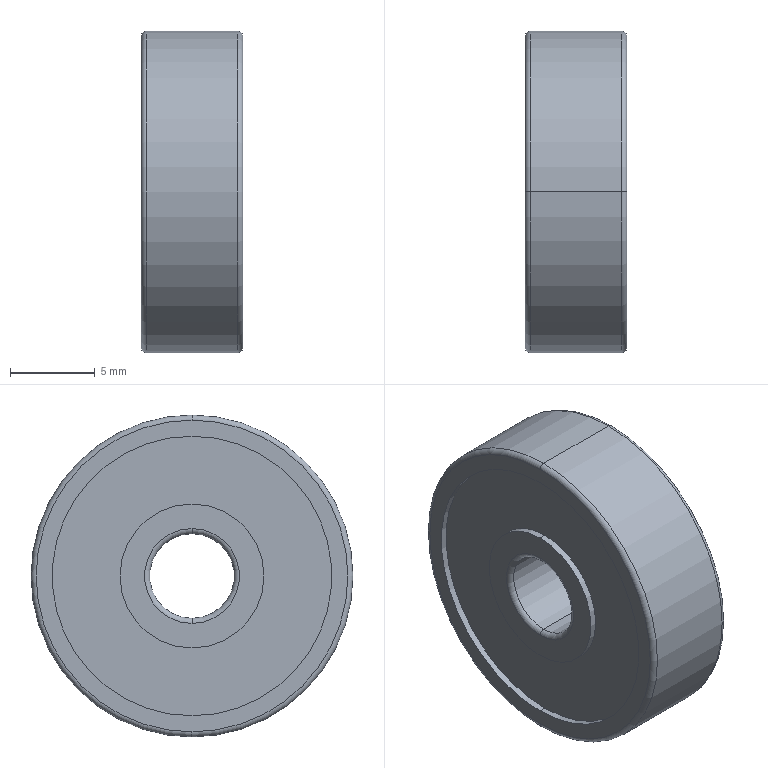Part | SolidWorks | features RefAxis 6, 3DProfileFeature 2, Revolution 1 | 1 solid | 26 faces | box 6 x 19 x 19 mm | volume 1455 mm3 | cylinder 12 | torus 8 | plane 6 | commonest cylinder face diameters 8.5 x4 16.5 x4 5 x2 19 x2
STEP:
#1=CARTESIAN_POINT('',(5.7,0.,9.5));
#2=VERTEX_POINT('',#1);
#3=CARTESIAN_POINT('',(5.7,0.,-9.5));
#4=VERTEX_POINT('',#3);
#5=CARTESIAN_POINT('',(5.7,0.,0.));
#6=DIRECTION('',(-1.,0.,0.));
#7=DIRECTION('',(0.,0.,1.));
#8=AXIS2_PLACEMENT_3D('',#5,#6,#7);
#9=CIRCLE('',#8,9.5);
#10=EDGE_CURVE('',#2,#4,#9,.T.);
#11=ORIENTED_EDGE('',*,*,#10,.T.);
#12=CARTESIAN_POINT('',(0.3,0.,-9.5));
#13=VERTEX_POINT('',#12);
#14=CARTESIAN_POINT('',(5.7,0.,-9.5));
#15=DIRECTION('',(-1.,0.,0.));
#16=VECTOR('',#15,1000.);
#17=LINE('',#14,#16);
#18=EDGE_CURVE('',#4,#13,#17,.T.);
#19=ORIENTED_EDGE('',*,*,#18,.T.);
#20=CARTESIAN_POINT('',(0.3,0.,9.5));
#21=VERTEX_POINT('',#20);
#22=CARTESIAN_POINT('',(0.3,0.,0.));
#23=DIRECTION('',(-1.,0.,0.));
#24=DIRECTION('',(0.,0.,1.));
#25=AXIS2_PLACEMENT_3D('',#22,#23,#24);
#26=CIRCLE('',#25,9.5);
#27=EDGE_CURVE('',#21,#13,#26,.T.);
#28=ORIENTED_EDGE('',*,*,#27,.F.);
#29=CARTESIAN_POINT('',(5.7,0.,9.5));
#30=DIRECTION('',(-1.,0.,0.));
#31=VECTOR('',#30,1000.);
#32=LINE('',#29,#31);
#33=EDGE_CURVE('',#2,#21,#32,.T.);
#34=ORIENTED_EDGE('',*,*,#33,.F.);
#35=EDGE_LOOP('',(#11,#19,#28,#34));
#36=FACE_OUTER_BOUND('',#35,.T.);
#37=CARTESIAN_POINT('',(5.7,0.,0.));
#38=DIRECTION('',(-1.,0.,0.));
#39=DIRECTION('',(0.,0.,1.));
#40=AXIS2_PLACEMENT_3D('',#37,#38,#39);
#41=CYLINDRICAL_SURFACE('',#40,9.5);
#42=ADVANCED_FACE('',(#36),#41,.T.);
#43=CARTESIAN_POINT('',(6.,0.,9.2));
#44=VERTEX_POINT('',#43);
#45=CARTESIAN_POINT('',(6.,0.,-9.2));
#46=VERTEX_POINT('',#45);
#47=CARTESIAN_POINT('',(6.,0.,0.));
#48=DIRECTION('',(-1.,0.,0.));
#49=DIRECTION('',(0.,0.,1.));
#50=AXIS2_PLACEMENT_3D('',#47,#48,#49);
#51=CIRCLE('',#50,9.2);
#52=EDGE_CURVE('',#44,#46,#51,.T.);
#53=ORIENTED_EDGE('',*,*,#52,.T.);
#54=CARTESIAN_POINT('',(5.7,0.,-9.2));
#55=DIRECTION('',(0.,1.,0.));
#56=DIRECTION('',(0.,0.,1.));
#57=AXIS2_PLACEMENT_3D('',#54,#55,#56);
#58=CIRCLE('',#57,0.3);
#59=EDGE_CURVE('',#46,#4,#58,.T.);
#60=ORIENTED_EDGE('',*,*,#59,.T.);
#61=ORIENTED_EDGE('',*,*,#10,.F.);
#62=CARTESIAN_POINT('',(5.7,0.,9.2));
#63=DIRECTION('',(0.,-1.,0.));
#64=DIRECTION('',(0.,0.,-1.));
#65=AXIS2_PLACEMENT_3D('',#62,#63,#64);
#66=CIRCLE('',#65,0.3);
#67=EDGE_CURVE('',#44,#2,#66,.T.);
#68=ORIENTED_EDGE('',*,*,#67,.F.);
#69=EDGE_LOOP('',(#53,#60,#61,#68));
#70=FACE_OUTER_BOUND('',#69,.T.);
#71=CARTESIAN_POINT('',(5.7,0.,0.));
#72=DIRECTION('',(-1.,0.,0.));
#73=DIRECTION('',(0.,0.,1.));
#74=AXIS2_PLACEMENT_3D('',#71,#72,#73);
#75=TOROIDAL_SURFACE('',#74,9.2,0.3);
#76=ADVANCED_FACE('',(#70),#75,.T.);
#77=CARTESIAN_POINT('',(6.,0.,-8.25));
#78=VERTEX_POINT('',#77);
#79=CARTESIAN_POINT('',(6.,0.,8.25));
#80=VERTEX_POINT('',#79);
#81=CARTESIAN_POINT('',(6.,0.,0.));
#82=DIRECTION('',(-1.,0.,0.));
#83=DIRECTION('',(0.,0.,1.));
#84=AXIS2_PLACEMENT_3D('',#81,#82,#83);
#85=CIRCLE('',#84,8.25);
#86=EDGE_CURVE('',#78,#80,#85,.T.);
#87=ORIENTED_EDGE('',*,*,#86,.F.);
#88=CARTESIAN_POINT('',(5.602,0.,-8.25));
#89=VERTEX_POINT('',#88);
#90=CARTESIAN_POINT('',(5.7,0.,-8.25));
#91=DIRECTION('',(-1.,0.,0.));
#92=VECTOR('',#91,1000.);
#93=LINE('',#90,#92);
#94=EDGE_CURVE('',#78,#89,#93,.T.);
#95=ORIENTED_EDGE('',*,*,#94,.T.);
#96=CARTESIAN_POINT('',(5.602,0.,8.25));
#97=VERTEX_POINT('',#96);
#98=CARTESIAN_POINT('',(5.602,0.,0.));
#99=DIRECTION('',(-1.,0.,0.));
#100=DIRECTION('',(0.,0.,1.));
#101=AXIS2_PLACEMENT_3D('',#98,#99,#100);
#102=CIRCLE('',#101,8.25);
#103=EDGE_CURVE('',#89,#97,#102,.T.);
#104=ORIENTED_EDGE('',*,*,#103,.T.);
#105=CARTESIAN_POINT('',(5.7,0.,8.25));
#106=DIRECTION('',(-1.,0.,0.));
#107=VECTOR('',#106,1000.);
#108=LINE('',#105,#107);
#109=EDGE_CURVE('',#80,#97,#108,.T.);
#110=ORIENTED_EDGE('',*,*,#109,.F.);
#111=EDGE_LOOP('',(#87,#95,#104,#110));
#112=FACE_OUTER_BOUND('',#111,.T.);
#113=CARTESIAN_POINT('',(5.7,0.,0.));
#114=DIRECTION('',(-1.,0.,0.));
#115=DIRECTION('',(0.,0.,1.));
#116=AXIS2_PLACEMENT_3D('',#113,#114,#115);
#117=CYLINDRICAL_SURFACE('',#116,8.25);
#118=ADVANCED_FACE('',(#112),#117,.F.);
#119=CARTESIAN_POINT('',(6.,0.,4.25));
#120=VERTEX_POINT('',#119);
#121=CARTESIAN_POINT('',(6.,0.,-4.25));
#122=VERTEX_POINT('',#121);
#123=CARTESIAN_POINT('',(6.,0.,0.));
#124=DIRECTION('',(-1.,0.,0.));
#125=DIRECTION('',(0.,0.,1.));
#126=AXIS2_PLACEMENT_3D('',#123,#124,#125);
#127=CIRCLE('',#126,4.25);
#128=EDGE_CURVE('',#120,#122,#127,.T.);
#129=ORIENTED_EDGE('',*,*,#128,.T.);
#130=CARTESIAN_POINT('',(5.602,0.,-4.25));
#131=VERTEX_POINT('',#130);
#132=CARTESIAN_POINT('',(5.7,0.,-4.25));
#133=DIRECTION('',(-1.,0.,0.));
#134=VECTOR('',#133,1000.);
#135=LINE('',#132,#134);
#136=EDGE_CURVE('',#122,#131,#135,.T.);
#137=ORIENTED_EDGE('',*,*,#136,.T.);
#138=CARTESIAN_POINT('',(5.602,0.,4.25));
#139=VERTEX_POINT('',#138);
#140=CARTESIAN_POINT('',(5.602,0.,0.));
#141=DIRECTION('',(-1.,0.,0.));
#142=DIRECTION('',(0.,0.,1.));
#143=AXIS2_PLACEMENT_3D('',#140,#141,#142);
#144=CIRCLE('',#143,4.25);
#145=EDGE_CURVE('',#139,#131,#144,.T.);
#146=ORIENTED_EDGE('',*,*,#145,.F.);
#147=CARTESIAN_POINT('',(5.7,0.,4.25));
#148=DIRECTION('',(-1.,0.,0.));
#149=VECTOR('',#148,1000.);
#150=LINE('',#147,#149);
#151=EDGE_CURVE('',#120,#139,#150,.T.);
#152=ORIENTED_EDGE('',*,*,#151,.F.);
#153=EDGE_LOOP('',(#129,#137,#146,#152));
#154=FACE_OUTER_BOUND('',#153,.T.);
#155=CARTESIAN_POINT('',(5.7,0.,0.));
#156=DIRECTION('',(-1.,0.,0.));
#157=DIRECTION('',(0.,0.,1.));
#158=AXIS2_PLACEMENT_3D('',#155,#156,#157);
#159=CYLINDRICAL_SURFACE('',#158,4.25);
#160=ADVANCED_FACE('',(#154),#159,.T.);
#161=CARTESIAN_POINT('',(5.7,0.,2.5));
#162=VERTEX_POINT('',#161);
#163=CARTESIAN_POINT('',(5.7,0.,-2.5));
#164=VERTEX_POINT('',#163);
#165=CARTESIAN_POINT('',(5.7,0.,0.));
#166=DIRECTION('',(-1.,0.,0.));
#167=DIRECTION('',(0.,0.,1.));
#168=AXIS2_PLACEMENT_3D('',#165,#166,#167);
#169=CIRCLE('',#168,2.5);
#170=EDGE_CURVE('',#162,#164,#169,.T.);
#171=ORIENTED_EDGE('',*,*,#170,.T.);
#172=CARTESIAN_POINT('',(6.,0.,-2.8));
#173=VERTEX_POINT('',#172);
#174=CARTESIAN_POINT('',(5.7,0.,-2.8));
#175=DIRECTION('',(0.,1.,0.));
#176=DIRECTION('',(0.,0.,1.));
#177=AXIS2_PLACEMENT_3D('',#174,#175,#176);
#178=CIRCLE('',#177,0.3);
#179=EDGE_CURVE('',#164,#173,#178,.T.);
#180=ORIENTED_EDGE('',*,*,#179,.T.);
#181=CARTESIAN_POINT('',(6.,0.,2.8));
#182=VERTEX_POINT('',#181);
#183=CARTESIAN_POINT('',(6.,0.,0.));
#184=DIRECTION('',(-1.,0.,0.));
#185=DIRECTION('',(0.,0.,1.));
#186=AXIS2_PLACEMENT_3D('',#183,#184,#185);
#187=CIRCLE('',#186,2.8);
#188=EDGE_CURVE('',#182,#173,#187,.T.);
#189=ORIENTED_EDGE('',*,*,#188,.F.);
#190=CARTESIAN_POINT('',(5.7,0.,2.8));
#191=DIRECTION('',(0.,-1.,0.));
#192=DIRECTION('',(0.,0.,-1.));
#193=AXIS2_PLACEMENT_3D('',#190,#191,#192);
#194=CIRCLE('',#193,0.3);
#195=EDGE_CURVE('',#162,#182,#194,.T.);
#196=ORIENTED_EDGE('',*,*,#195,.F.);
#197=EDGE_LOOP('',(#171,#180,#189,#196));
#198=FACE_OUTER_BOUND('',#197,.T.);
#199=CARTESIAN_POINT('',(5.7,0.,0.));
#200=DIRECTION('',(-1.,0.,0.));
#201=DIRECTION('',(0.,0.,1.));
#202=AXIS2_PLACEMENT_3D('',#199,#200,#201);
#203=TOROIDAL_SURFACE('',#202,2.8,0.3);
#204=ADVANCED_FACE('',(#198),#203,.T.);
#205=CARTESIAN_POINT('',(5.7,0.,0.));
#206=DIRECTION('',(-1.,0.,0.));
#207=DIRECTION('',(0.,0.,1.));
#208=AXIS2_PLACEMENT_3D('',#205,#206,#207);
#209=CIRCLE('',#208,2.5);
#210=EDGE_CURVE('',#164,#162,#209,.T.);
#211=ORIENTED_EDGE('',*,*,#210,.F.);
#212=CARTESIAN_POINT('',(0.3,0.,-2.5));
#213=VERTEX_POINT('',#212);
#214=CARTESIAN_POINT('',(5.7,0.,-2.5));
#215=DIRECTION('',(-1.,0.,0.));
#216=VECTOR('',#215,1000.);
#217=LINE('',#214,#216);
#218=EDGE_CURVE('',#164,#213,#217,.T.);
#219=ORIENTED_EDGE('',*,*,#218,.T.);
#220=CARTESIAN_POINT('',(0.3,0.,2.5));
#221=VERTEX_POINT('',#220);
#222=CARTESIAN_POINT('',(0.3,0.,0.));
#223=DIRECTION('',(-1.,0.,0.));
#224=DIRECTION('',(0.,0.,1.));
#225=AXIS2_PLACEMENT_3D('',#222,#223,#224);
#226=CIRCLE('',#225,2.5);
#227=EDGE_CURVE('',#213,#221,#226,.T.);
#228=ORIENTED_EDGE('',*,*,#227,.T.);
#229=CARTESIAN_POINT('',(5.7,0.,2.5));
#230=DIRECTION('',(-1.,0.,0.));
#231=VECTOR('',#230,1000.);
#232=LINE('',#229,#231);
#233=EDGE_CURVE('',#162,#221,#232,.T.);
#234=ORIENTED_EDGE('',*,*,#233,.F.);
#235=EDGE_LOOP('',(#211,#219,#228,#234));
#236=FACE_OUTER_BOUND('',#235,.T.);
#237=CARTESIAN_POINT('',(5.7,0.,0.));
#238=DIRECTION('',(-1.,0.,0.));
#239=DIRECTION('',(0.,0.,1.));
#240=AXIS2_PLACEMENT_3D('',#237,#238,#239);
#241=CYLINDRICAL_SURFACE('',#240,2.5);
#242=ADVANCED_FACE('',(#236),#241,.F.);
#243=CARTESIAN_POINT('',(0.,0.,2.8));
#244=VERTEX_POINT('',#243);
#245=CARTESIAN_POINT('',(0.,0.,-2.8));
#246=VERTEX_POINT('',#245);
#247=CARTESIAN_POINT('',(0.,0.,0.));
#248=DIRECTION('',(-1.,0.,0.));
#249=DIRECTION('',(0.,0.,1.));
#250=AXIS2_PLACEMENT_3D('',#247,#248,#249);
#251=CIRCLE('',#250,2.8);
#252=EDGE_CURVE('',#244,#246,#251,.T.);
#253=ORIENTED_EDGE('',*,*,#252,.T.);
#254=CARTESIAN_POINT('',(0.3,0.,-2.8));
#255=DIRECTION('',(0.,1.,0.));
#256=DIRECTION('',(0.,0.,1.));
#257=AXIS2_PLACEMENT_3D('',#254,#255,#256);
#258=CIRCLE('',#257,0.3);
#259=EDGE_CURVE('',#246,#213,#258,.T.);
#260=ORIENTED_EDGE('',*,*,#259,.T.);
#261=CARTESIAN_POINT('',(0.3,0.,0.));
#262=DIRECTION('',(-1.,0.,0.));
#263=DIRECTION('',(0.,0.,1.));
#264=AXIS2_PLACEMENT_3D('',#261,#262,#263);
#265=CIRCLE('',#264,2.5);
#266=EDGE_CURVE('',#221,#213,#265,.T.);
#267=ORIENTED_EDGE('',*,*,#266,.F.);
#268=CARTESIAN_POINT('',(0.3,0.,2.8));
#269=DIRECTION('',(0.,-1.,0.));
#270=DIRECTION('',(0.,0.,-1.));
#271=AXIS2_PLACEMENT_3D('',#268,#269,#270);
#272=CIRCLE('',#271,0.3);
#273=EDGE_CURVE('',#244,#221,#272,.T.);
#274=ORIENTED_EDGE('',*,*,#273,.F.);
#275=EDGE_LOOP('',(#253,#260,#267,#274));
#276=FACE_OUTER_BOUND('',#275,.T.);
#277=CARTESIAN_POINT('',(0.3,0.,0.));
#278=DIRECTION('',(-1.,0.,0.));
#279=DIRECTION('',(0.,0.,1.));
#280=AXIS2_PLACEMENT_3D('',#277,#278,#279);
#281=TOROIDAL_SURFACE('',#280,2.8,0.3);
#282=ADVANCED_FACE('',(#276),#281,.T.);
#283=CARTESIAN_POINT('',(0.3984,0.,4.25));
#284=VERTEX_POINT('',#283);
#285=CARTESIAN_POINT('',(0.3984,0.,-4.25));
#286=VERTEX_POINT('',#285);
#287=CARTESIAN_POINT('',(0.3984,0.,0.));
#288=DIRECTION('',(-1.,0.,0.));
#289=DIRECTION('',(0.,0.,1.));
#290=AXIS2_PLACEMENT_3D('',#287,#288,#289);
#291=CIRCLE('',#290,4.25);
#292=EDGE_CURVE('',#284,#286,#291,.T.);
#293=ORIENTED_EDGE('',*,*,#292,.T.);
#294=CARTESIAN_POINT('',(0.,0.,-4.25));
#295=VERTEX_POINT('',#294);
#296=CARTESIAN_POINT('',(5.7,0.,-4.25));
#297=DIRECTION('',(-1.,0.,0.));
#298=VECTOR('',#297,1000.);
#299=LINE('',#296,#298);
#300=EDGE_CURVE('',#286,#295,#299,.T.);
#301=ORIENTED_EDGE('',*,*,#300,.T.);
#302=CARTESIAN_POINT('',(0.,0.,4.25));
#303=VERTEX_POINT('',#302);
#304=CARTESIAN_POINT('',(0.,0.,0.));
#305=DIRECTION('',(-1.,0.,0.));
#306=DIRECTION('',(0.,0.,1.));
#307=AXIS2_PLACEMENT_3D('',#304,#305,#306);
#308=CIRCLE('',#307,4.25);
#309=EDGE_CURVE('',#303,#295,#308,.T.);
#310=ORIENTED_EDGE('',*,*,#309,.F.);
#311=CARTESIAN_POINT('',(5.7,0.,4.25));
#312=DIRECTION('',(-1.,0.,0.));
#313=VECTOR('',#312,1000.);
#314=LINE('',#311,#313);
#315=EDGE_CURVE('',#284,#303,#314,.T.);
#316=ORIENTED_EDGE('',*,*,#315,.F.);
#317=EDGE_LOOP('',(#293,#301,#310,#316));
#318=FACE_OUTER_BOUND('',#317,.T.);
#319=CARTESIAN_POINT('',(5.7,0.,0.));
#320=DIRECTION('',(-1.,0.,0.));
#321=DIRECTION('',(0.,0.,1.));
#322=AXIS2_PLACEMENT_3D('',#319,#320,#321);
#323=CYLINDRICAL_SURFACE('',#322,4.25);
#324=ADVANCED_FACE('',(#318),#323,.T.);
#325=CARTESIAN_POINT('',(0.3984,0.,-8.25));
#326=VERTEX_POINT('',#325);
#327=CARTESIAN_POINT('',(0.3984,0.,8.25));
#328=VERTEX_POINT('',#327);
#329=CARTESIAN_POINT('',(0.3984,0.,0.));
#330=DIRECTION('',(-1.,0.,0.));
#331=DIRECTION('',(0.,0.,1.));
#332=AXIS2_PLACEMENT_3D('',#329,#330,#331);
#333=CIRCLE('',#332,8.25);
#334=EDGE_CURVE('',#326,#328,#333,.T.);
#335=ORIENTED_EDGE('',*,*,#334,.F.);
#336=CARTESIAN_POINT('',(0.,0.,-8.25));
#337=VERTEX_POINT('',#336);
#338=CARTESIAN_POINT('',(5.7,0.,-8.25));
#339=DIRECTION('',(-1.,0.,0.));
#340=VECTOR('',#339,1000.);
#341=LINE('',#338,#340);
#342=EDGE_CURVE('',#326,#337,#341,.T.);
#343=ORIENTED_EDGE('',*,*,#342,.T.);
#344=CARTESIAN_POINT('',(0.,0.,8.25));
#345=VERTEX_POINT('',#344);
#346=CARTESIAN_POINT('',(0.,0.,0.));
#347=DIRECTION('',(-1.,0.,0.));
#348=DIRECTION('',(0.,0.,1.));
#349=AXIS2_PLACEMENT_3D('',#346,#347,#348);
#350=CIRCLE('',#349,8.25);
#351=EDGE_CURVE('',#337,#345,#350,.T.);
#352=ORIENTED_EDGE('',*,*,#351,.T.);
#353=CARTESIAN_POINT('',(5.7,0.,8.25));
#354=DIRECTION('',(-1.,0.,0.));
#355=VECTOR('',#354,1000.);
#356=LINE('',#353,#355);
#357=EDGE_CURVE('',#328,#345,#356,.T.);
#358=ORIENTED_EDGE('',*,*,#357,.F.);
#359=EDGE_LOOP('',(#335,#343,#352,#358));
#360=FACE_OUTER_BOUND('',#359,.T.);
#361=CARTESIAN_POINT('',(5.7,0.,0.));
#362=DIRECTION('',(-1.,0.,0.));
#363=DIRECTION('',(0.,0.,1.));
#364=AXIS2_PLACEMENT_3D('',#361,#362,#363);
#365=CYLINDRICAL_SURFACE('',#364,8.25);
#366=ADVANCED_FACE('',(#360),#365,.F.);
#367=ORIENTED_EDGE('',*,*,#27,.T.);
#368=CARTESIAN_POINT('',(0.,0.,-9.2));
#369=VERTEX_POINT('',#368);
#370=CARTESIAN_POINT('',(0.3,0.,-9.2));
#371=DIRECTION('',(0.,1.,0.));
#372=DIRECTION('',(0.,0.,1.));
#373=AXIS2_PLACEMENT_3D('',#370,#371,#372);
#374=CIRCLE('',#373,0.3);
#375=EDGE_CURVE('',#13,#369,#374,.T.);
#376=ORIENTED_EDGE('',*,*,#375,.T.);
#377=CARTESIAN_POINT('',(0.,0.,9.2));
#378=VERTEX_POINT('',#377);
#379=CARTESIAN_POINT('',(0.,0.,0.));
#380=DIRECTION('',(-1.,0.,0.));
#381=DIRECTION('',(0.,0.,1.));
#382=AXIS2_PLACEMENT_3D('',#379,#380,#381);
#383=CIRCLE('',#382,9.2);
#384=EDGE_CURVE('',#378,#369,#383,.T.);
#385=ORIENTED_EDGE('',*,*,#384,.F.);
#386=CARTESIAN_POINT('',(0.3,0.,9.2));
#387=DIRECTION('',(0.,-1.,0.));
#388=DIRECTION('',(0.,0.,-1.));
#389=AXIS2_PLACEMENT_3D('',#386,#387,#388);
#390=CIRCLE('',#389,0.3);
#391=EDGE_CURVE('',#21,#378,#390,.T.);
#392=ORIENTED_EDGE('',*,*,#391,.F.);
#393=EDGE_LOOP('',(#367,#376,#385,#392));
#394=FACE_OUTER_BOUND('',#393,.T.);
#395=CARTESIAN_POINT('',(0.3,0.,0.));
#396=DIRECTION('',(-1.,0.,0.));
#397=DIRECTION('',(0.,0.,1.));
#398=AXIS2_PLACEMENT_3D('',#395,#396,#397);
#399=TOROIDAL_SURFACE('',#398,9.2,0.3);
#400=ADVANCED_FACE('',(#394),#399,.T.);
#401=ORIENTED_EDGE('',*,*,#375,.F.);
#402=CARTESIAN_POINT('',(0.3,0.,0.));
#403=DIRECTION('',(-1.,0.,0.));
#404=DIRECTION('',(0.,0.,1.));
#405=AXIS2_PLACEMENT_3D('',#402,#403,#404);
#406=CIRCLE('',#405,9.5);
#407=EDGE_CURVE('',#13,#21,#406,.T.);
#408=ORIENTED_EDGE('',*,*,#407,.T.);
#409=ORIENTED_EDGE('',*,*,#391,.T.);
#410=CARTESIAN_POINT('',(0.,0.,0.));
#411=DIRECTION('',(-1.,0.,0.));
#412=DIRECTION('',(0.,0.,1.));
#413=AXIS2_PLACEMENT_3D('',#410,#411,#412);
#414=CIRCLE('',#413,9.2);
#415=EDGE_CURVE('',#369,#378,#414,.T.);
#416=ORIENTED_EDGE('',*,*,#415,.F.);
#417=EDGE_LOOP('',(#401,#408,#409,#416));
#418=FACE_OUTER_BOUND('',#417,.T.);
#419=CARTESIAN_POINT('',(0.3,0.,0.));
#420=DIRECTION('',(-1.,0.,0.));
#421=DIRECTION('',(0.,0.,1.));
#422=AXIS2_PLACEMENT_3D('',#419,#420,#421);
#423=TOROIDAL_SURFACE('',#422,9.2,0.3);
#424=ADVANCED_FACE('',(#418),#423,.T.);
#425=CARTESIAN_POINT('',(0.,0.,0.));
#426=DIRECTION('',(-1.,0.,0.));
#427=DIRECTION('',(0.,0.,1.));
#428=AXIS2_PLACEMENT_3D('',#425,#426,#427);
#429=CIRCLE('',#428,8.25);
#430=EDGE_CURVE('',#345,#337,#429,.T.);
#431=ORIENTED_EDGE('',*,*,#430,.F.);
#432=ORIENTED_EDGE('',*,*,#351,.F.);
#433=EDGE_LOOP('',(#431,#432));
#434=FACE_BOUND('',#433,.T.);
#435=ORIENTED_EDGE('',*,*,#384,.T.);
#436=ORIENTED_EDGE('',*,*,#415,.T.);
#437=EDGE_LOOP('',(#435,#436));
#438=FACE_OUTER_BOUND('',#437,.T.);
#439=CARTESIAN_POINT('',(0.,9.2,0.));
#440=DIRECTION('',(1.,0.,0.));
#441=DIRECTION('',(0.,0.,-1.));
#442=AXIS2_PLACEMENT_3D('',#439,#440,#441);
#443=PLANE('',#442);
#444=ADVANCED_FACE('',(#434,#438),#443,.F.);
#445=ORIENTED_EDGE('',*,*,#342,.F.);
#446=CARTESIAN_POINT('',(0.3984,0.,0.));
#447=DIRECTION('',(-1.,0.,0.));
#448=DIRECTION('',(0.,0.,1.));
#449=AXIS2_PLACEMENT_3D('',#446,#447,#448);
#450=CIRCLE('',#449,8.25);
#451=EDGE_CURVE('',#328,#326,#450,.T.);
#452=ORIENTED_EDGE('',*,*,#451,.F.);
#453=ORIENTED_EDGE('',*,*,#357,.T.);
#454=ORIENTED_EDGE('',*,*,#430,.T.);
#455=EDGE_LOOP('',(#445,#452,#453,#454));
#456=FACE_OUTER_BOUND('',#455,.T.);
#457=CARTESIAN_POINT('',(5.7,0.,0.));
#458=DIRECTION('',(-1.,0.,0.));
#459=DIRECTION('',(0.,0.,1.));
#460=AXIS2_PLACEMENT_3D('',#457,#458,#459);
#461=CYLINDRICAL_SURFACE('',#460,8.25);
#462=ADVANCED_FACE('',(#456),#461,.F.);
#463=ORIENTED_EDGE('',*,*,#292,.F.);
#464=CARTESIAN_POINT('',(0.3984,0.,0.));
#465=DIRECTION('',(-1.,0.,0.));
#466=DIRECTION('',(0.,0.,1.));
#467=AXIS2_PLACEMENT_3D('',#464,#465,#466);
#468=CIRCLE('',#467,4.25);
#469=EDGE_CURVE('',#286,#284,#468,.T.);
#470=ORIENTED_EDGE('',*,*,#469,.F.);
#471=EDGE_LOOP('',(#463,#470));
#472=FACE_BOUND('',#471,.T.);
#473=ORIENTED_EDGE('',*,*,#451,.T.);
#474=ORIENTED_EDGE('',*,*,#334,.T.);
#475=EDGE_LOOP('',(#473,#474));
#476=FACE_OUTER_BOUND('',#475,.T.);
#477=CARTESIAN_POINT('',(0.3984,8.25,0.));
#478=DIRECTION('',(1.,0.,0.));
#479=DIRECTION('',(0.,0.,-1.));
#480=AXIS2_PLACEMENT_3D('',#477,#478,#479);
#481=PLANE('',#480);
#482=ADVANCED_FACE('',(#472,#476),#481,.F.);
#483=ORIENTED_EDGE('',*,*,#300,.F.);
#484=ORIENTED_EDGE('',*,*,#469,.T.);
#485=ORIENTED_EDGE('',*,*,#315,.T.);
#486=CARTESIAN_POINT('',(0.,0.,0.));
#487=DIRECTION('',(-1.,0.,0.));
#488=DIRECTION('',(0.,0.,1.));
#489=AXIS2_PLACEMENT_3D('',#486,#487,#488);
#490=CIRCLE('',#489,4.25);
#491=EDGE_CURVE('',#295,#303,#490,.T.);
#492=ORIENTED_EDGE('',*,*,#491,.F.);
#493=EDGE_LOOP('',(#483,#484,#485,#492));
#494=FACE_OUTER_BOUND('',#493,.T.);
#495=CARTESIAN_POINT('',(5.7,0.,0.));
#496=DIRECTION('',(-1.,0.,0.));
#497=DIRECTION('',(0.,0.,1.));
#498=AXIS2_PLACEMENT_3D('',#495,#496,#497);
#499=CYLINDRICAL_SURFACE('',#498,4.25);
#500=ADVANCED_FACE('',(#494),#499,.T.);
#501=ORIENTED_EDGE('',*,*,#252,.F.);
#502=CARTESIAN_POINT('',(0.,0.,0.));
#503=DIRECTION('',(-1.,0.,0.));
#504=DIRECTION('',(0.,0.,1.));
#505=AXIS2_PLACEMENT_3D('',#502,#503,#504);
#506=CIRCLE('',#505,2.8);
#507=EDGE_CURVE('',#246,#244,#506,.T.);
#508=ORIENTED_EDGE('',*,*,#507,.F.);
#509=EDGE_LOOP('',(#501,#508));
#510=FACE_BOUND('',#509,.T.);
#511=ORIENTED_EDGE('',*,*,#309,.T.);
#512=ORIENTED_EDGE('',*,*,#491,.T.);
#513=EDGE_LOOP('',(#511,#512));
#514=FACE_OUTER_BOUND('',#513,.T.);
#515=CARTESIAN_POINT('',(0.,4.25,0.));
#516=DIRECTION('',(1.,0.,0.));
#517=DIRECTION('',(0.,0.,-1.));
#518=AXIS2_PLACEMENT_3D('',#515,#516,#517);
#519=PLANE('',#518);
#520=ADVANCED_FACE('',(#510,#514),#519,.F.);
#521=ORIENTED_EDGE('',*,*,#259,.F.);
#522=ORIENTED_EDGE('',*,*,#507,.T.);
#523=ORIENTED_EDGE('',*,*,#273,.T.);
#524=ORIENTED_EDGE('',*,*,#227,.F.);
#525=EDGE_LOOP('',(#521,#522,#523,#524));
#526=FACE_OUTER_BOUND('',#525,.T.);
#527=CARTESIAN_POINT('',(0.3,0.,0.));
#528=DIRECTION('',(-1.,0.,0.));
#529=DIRECTION('',(0.,0.,1.));
#530=AXIS2_PLACEMENT_3D('',#527,#528,#529);
#531=TOROIDAL_SURFACE('',#530,2.8,0.3);
#532=ADVANCED_FACE('',(#526),#531,.T.);
#533=ORIENTED_EDGE('',*,*,#218,.F.);
#534=ORIENTED_EDGE('',*,*,#170,.F.);
#535=ORIENTED_EDGE('',*,*,#233,.T.);
#536=ORIENTED_EDGE('',*,*,#266,.T.);
#537=EDGE_LOOP('',(#533,#534,#535,#536));
#538=FACE_OUTER_BOUND('',#537,.T.);
#539=CARTESIAN_POINT('',(5.7,0.,0.));
#540=DIRECTION('',(-1.,0.,0.));
#541=DIRECTION('',(0.,0.,1.));
#542=AXIS2_PLACEMENT_3D('',#539,#540,#541);
#543=CYLINDRICAL_SURFACE('',#542,2.5);
#544=ADVANCED_FACE('',(#538),#543,.F.);
#545=ORIENTED_EDGE('',*,*,#179,.F.);
#546=ORIENTED_EDGE('',*,*,#210,.T.);
#547=ORIENTED_EDGE('',*,*,#195,.T.);
#548=CARTESIAN_POINT('',(6.,0.,0.));
#549=DIRECTION('',(-1.,0.,0.));
#550=DIRECTION('',(0.,0.,1.));
#551=AXIS2_PLACEMENT_3D('',#548,#549,#550);
#552=CIRCLE('',#551,2.8);
#553=EDGE_CURVE('',#173,#182,#552,.T.);
#554=ORIENTED_EDGE('',*,*,#553,.F.);
#555=EDGE_LOOP('',(#545,#546,#547,#554));
#556=FACE_OUTER_BOUND('',#555,.T.);
#557=CARTESIAN_POINT('',(5.7,0.,0.));
#558=DIRECTION('',(-1.,0.,0.));
#559=DIRECTION('',(0.,0.,1.));
#560=AXIS2_PLACEMENT_3D('',#557,#558,#559);
#561=TOROIDAL_SURFACE('',#560,2.8,0.3);
#562=ADVANCED_FACE('',(#556),#561,.T.);
#563=ORIENTED_EDGE('',*,*,#128,.F.);
#564=CARTESIAN_POINT('',(6.,0.,0.));
#565=DIRECTION('',(-1.,0.,0.));
#566=DIRECTION('',(0.,0.,1.));
#567=AXIS2_PLACEMENT_3D('',#564,#565,#566);
#568=CIRCLE('',#567,4.25);
#569=EDGE_CURVE('',#122,#120,#568,.T.);
#570=ORIENTED_EDGE('',*,*,#569,.F.);
#571=EDGE_LOOP('',(#563,#570));
#572=FACE_OUTER_BOUND('',#571,.T.);
#573=ORIENTED_EDGE('',*,*,#188,.T.);
#574=ORIENTED_EDGE('',*,*,#553,.T.);
#575=EDGE_LOOP('',(#573,#574));
#576=FACE_BOUND('',#575,.T.);
#577=CARTESIAN_POINT('',(6.,2.8,0.));
#578=DIRECTION('',(-1.,0.,0.));
#579=DIRECTION('',(0.,0.,1.));
#580=AXIS2_PLACEMENT_3D('',#577,#578,#579);
#581=PLANE('',#580);
#582=ADVANCED_FACE('',(#572,#576),#581,.F.);
#583=ORIENTED_EDGE('',*,*,#136,.F.);
#584=ORIENTED_EDGE('',*,*,#569,.T.);
#585=ORIENTED_EDGE('',*,*,#151,.T.);
#586=CARTESIAN_POINT('',(5.602,0.,0.));
#587=DIRECTION('',(-1.,0.,0.));
#588=DIRECTION('',(0.,0.,1.));
#589=AXIS2_PLACEMENT_3D('',#586,#587,#588);
#590=CIRCLE('',#589,4.25);
#591=EDGE_CURVE('',#131,#139,#590,.T.);
#592=ORIENTED_EDGE('',*,*,#591,.F.);
#593=EDGE_LOOP('',(#583,#584,#585,#592));
#594=FACE_OUTER_BOUND('',#593,.T.);
#595=CARTESIAN_POINT('',(5.7,0.,0.));
#596=DIRECTION('',(-1.,0.,0.));
#597=DIRECTION('',(0.,0.,1.));
#598=AXIS2_PLACEMENT_3D('',#595,#596,#597);
#599=CYLINDRICAL_SURFACE('',#598,4.25);
#600=ADVANCED_FACE('',(#594),#599,.T.);
#601=CARTESIAN_POINT('',(5.602,0.,0.));
#602=DIRECTION('',(-1.,0.,0.));
#603=DIRECTION('',(0.,0.,1.));
#604=AXIS2_PLACEMENT_3D('',#601,#602,#603);
#605=CIRCLE('',#604,8.25);
#606=EDGE_CURVE('',#97,#89,#605,.T.);
#607=ORIENTED_EDGE('',*,*,#606,.F.);
#608=ORIENTED_EDGE('',*,*,#103,.F.);
#609=EDGE_LOOP('',(#607,#608));
#610=FACE_OUTER_BOUND('',#609,.T.);
#611=ORIENTED_EDGE('',*,*,#145,.T.);
#612=ORIENTED_EDGE('',*,*,#591,.T.);
#613=EDGE_LOOP('',(#611,#612));
#614=FACE_BOUND('',#613,.T.);
#615=CARTESIAN_POINT('',(5.602,4.25,0.));
#616=DIRECTION('',(-1.,0.,0.));
#617=DIRECTION('',(0.,0.,1.));
#618=AXIS2_PLACEMENT_3D('',#615,#616,#617);
#619=PLANE('',#618);
#620=ADVANCED_FACE('',(#610,#614),#619,.F.);
#621=ORIENTED_EDGE('',*,*,#94,.F.);
#622=CARTESIAN_POINT('',(6.,0.,0.));
#623=DIRECTION('',(-1.,0.,0.));
#624=DIRECTION('',(0.,0.,1.));
#625=AXIS2_PLACEMENT_3D('',#622,#623,#624);
#626=CIRCLE('',#625,8.25);
#627=EDGE_CURVE('',#80,#78,#626,.T.);
#628=ORIENTED_EDGE('',*,*,#627,.F.);
#629=ORIENTED_EDGE('',*,*,#109,.T.);
#630=ORIENTED_EDGE('',*,*,#606,.T.);
#631=EDGE_LOOP('',(#621,#628,#629,#630));
#632=FACE_OUTER_BOUND('',#631,.T.);
#633=CARTESIAN_POINT('',(5.7,0.,0.));
#634=DIRECTION('',(-1.,0.,0.));
#635=DIRECTION('',(0.,0.,1.));
#636=AXIS2_PLACEMENT_3D('',#633,#634,#635);
#637=CYLINDRICAL_SURFACE('',#636,8.25);
#638=ADVANCED_FACE('',(#632),#637,.F.);
#639=ORIENTED_EDGE('',*,*,#52,.F.);
#640=CARTESIAN_POINT('',(6.,0.,0.));
#641=DIRECTION('',(-1.,0.,0.));
#642=DIRECTION('',(0.,0.,1.));
#643=AXIS2_PLACEMENT_3D('',#640,#641,#642);
#644=CIRCLE('',#643,9.2);
#645=EDGE_CURVE('',#46,#44,#644,.T.);
#646=ORIENTED_EDGE('',*,*,#645,.F.);
#647=EDGE_LOOP('',(#639,#646));
#648=FACE_OUTER_BOUND('',#647,.T.);
#649=ORIENTED_EDGE('',*,*,#627,.T.);
#650=ORIENTED_EDGE('',*,*,#86,.T.);
#651=EDGE_LOOP('',(#649,#650));
#652=FACE_BOUND('',#651,.T.);
#653=CARTESIAN_POINT('',(6.,8.25,0.));
#654=DIRECTION('',(-1.,0.,0.));
#655=DIRECTION('',(0.,0.,1.));
#656=AXIS2_PLACEMENT_3D('',#653,#654,#655);
#657=PLANE('',#656);
#658=ADVANCED_FACE('',(#648,#652),#657,.F.);
#659=ORIENTED_EDGE('',*,*,#59,.F.);
#660=ORIENTED_EDGE('',*,*,#645,.T.);
#661=ORIENTED_EDGE('',*,*,#67,.T.);
#662=CARTESIAN_POINT('',(5.7,0.,0.));
#663=DIRECTION('',(-1.,0.,0.));
#664=DIRECTION('',(0.,0.,1.));
#665=AXIS2_PLACEMENT_3D('',#662,#663,#664);
#666=CIRCLE('',#665,9.5);
#667=EDGE_CURVE('',#4,#2,#666,.T.);
#668=ORIENTED_EDGE('',*,*,#667,.F.);
#669=EDGE_LOOP('',(#659,#660,#661,#668));
#670=FACE_OUTER_BOUND('',#669,.T.);
#671=CARTESIAN_POINT('',(5.7,0.,0.));
#672=DIRECTION('',(-1.,0.,0.));
#673=DIRECTION('',(0.,0.,1.));
#674=AXIS2_PLACEMENT_3D('',#671,#672,#673);
#675=TOROIDAL_SURFACE('',#674,9.2,0.3);
#676=ADVANCED_FACE('',(#670),#675,.T.);
#677=ORIENTED_EDGE('',*,*,#18,.F.);
#678=ORIENTED_EDGE('',*,*,#667,.T.);
#679=ORIENTED_EDGE('',*,*,#33,.T.);
#680=ORIENTED_EDGE('',*,*,#407,.F.);
#681=EDGE_LOOP('',(#677,#678,#679,#680));
#682=FACE_OUTER_BOUND('',#681,.T.);
#683=CARTESIAN_POINT('',(5.7,0.,0.));
#684=DIRECTION('',(-1.,0.,0.));
#685=DIRECTION('',(0.,0.,1.));
#686=AXIS2_PLACEMENT_3D('',#683,#684,#685);
#687=CYLINDRICAL_SURFACE('',#686,9.5);
#688=ADVANCED_FACE('',(#682),#687,.T.);
#689=CLOSED_SHELL('',(#42,#76,#118,#160,#204,#242,#282,#324,#366,#400,#424,#444,#462,#482,#500,#520,#532,#544,#562,#582,#600,#620,#638,#658,#676,#688));
#690=MANIFOLD_SOLID_BREP('',#689);
#691=CARTESIAN_POINT('',(0.,0.,0.));
#692=DIRECTION('',(0.,0.,1.));
#693=DIRECTION('',(1.,0.,0.));
#694=AXIS2_PLACEMENT_3D('',#691,#692,#693);
#695=(LENGTH_UNIT()NAMED_UNIT(*)SI_UNIT(.MILLI.,.METRE.));
#696=UNCERTAINTY_MEASURE_WITH_UNIT(LENGTH_MEASURE(0.00001),#695,'','');
#697=(NAMED_UNIT(*)PLANE_ANGLE_UNIT()SI_UNIT($,.RADIAN.));
#698=(NAMED_UNIT(*)SI_UNIT($,.STERADIAN.)SOLID_ANGLE_UNIT());
#699=(GEOMETRIC_REPRESENTATION_CONTEXT(3)GLOBAL_UNCERTAINTY_ASSIGNED_CONTEXT((#696))GLOBAL_UNIT_ASSIGNED_CONTEXT((#695,#697,#698))REPRESENTATION_CONTEXT('',''));
#700=ADVANCED_BREP_SHAPE_REPRESENTATION('',(#690,#694),#699);